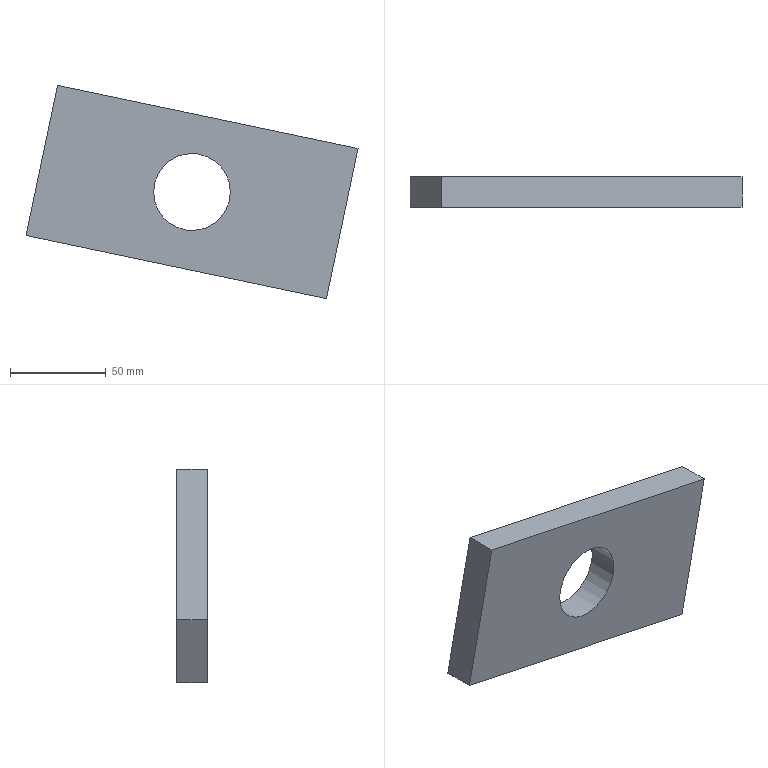Part | STEP file | 5_ESTAGIO_005 | 1 solid | 7 faces | box 173.032 x 16 x 111.193 mm | volume 184694 mm3 | plane 6 | cylinder 1 | commonest cylinder face diameters 40 x1
STEP:
#1=CARTESIAN_POINT('',(0.,0.,0.));
#2=DIRECTION('',(0.,0.,1.));
#3=DIRECTION('',(1.,0.,0.));
#4=AXIS2_PLACEMENT_3D('',#1,#2,#3);
#5=CARTESIAN_POINT('',(-2623.456,-962.15,953.739));
#6=VERTEX_POINT('',#5);
#7=CARTESIAN_POINT('',(-2641.008,-962.15,963.327));
#8=DIRECTION('',(0.,1.,0.));
#9=DIRECTION('',(1.,0.,0.));
#10=AXIS2_PLACEMENT_3D('',#7,#8,#9);
#11=CIRCLE('',#10,20.);
#12=CARTESIAN_POINT('',(-2641.008,-962.05,963.327));
#13=DIRECTION('',(0.,1.,0.));
#14=DIRECTION('',(0.8776,0.,-0.4794));
#15=AXIS2_PLACEMENT_3D('',#12,#13,#14);
#16=CYLINDRICAL_SURFACE('',#15,20.);
#17=CARTESIAN_POINT('',(-0.5,-0.1));
#18=DIRECTION('',(1.,0.));
#19=VECTOR('',#18,1.);
#20=LINE('',#17,#19);
#21=(GEOMETRIC_REPRESENTATION_CONTEXT(2)PARAMETRIC_REPRESENTATION_CONTEXT()REPRESENTATION_CONTEXT('',''));
#22=DEFINITIONAL_REPRESENTATION('',(#20),#21);
#23=PCURVE('',#16,#22);
#24=CARTESIAN_POINT('',(0.,-962.15,0.));
#25=DIRECTION('',(0.,1.,0.));
#26=DIRECTION('',(0.,0.,1.));
#27=AXIS2_PLACEMENT_3D('',#24,#25,#26);
#28=PLANE('',#27);
#29=CARTESIAN_POINT('',(963.327,-2641.008));
#30=DIRECTION('',(0.,1.));
#31=AXIS2_PLACEMENT_2D('',#29,#30);
#32=CIRCLE('',#31,20.);
#33=(GEOMETRIC_REPRESENTATION_CONTEXT(2)PARAMETRIC_REPRESENTATION_CONTEXT()REPRESENTATION_CONTEXT('',''));
#34=DEFINITIONAL_REPRESENTATION('',(#32),#33);
#35=PCURVE('',#28,#34);
#36=SURFACE_CURVE('',#11,(#23,#35),.PCURVE_S1.);
#37=EDGE_CURVE('',#6,#6,#36,.T.);
#38=ORIENTED_EDGE('',*,*,#37,.T.);
#39=CARTESIAN_POINT('',(-2623.456,-946.15,953.739));
#40=VERTEX_POINT('',#39);
#41=CARTESIAN_POINT('',(-2623.456,-962.15,953.739));
#42=CARTESIAN_POINT('',(-2623.456,-946.15,953.739));
#43=B_SPLINE_CURVE_WITH_KNOTS('',1,(#41,#42),.UNSPECIFIED.,.F.,.F.,(2,2),(-0.1,15.9),.PIECEWISE_BEZIER_KNOTS.);
#44=CARTESIAN_POINT('',(6.283,0.));
#45=DIRECTION('',(0.,1.));
#46=VECTOR('',#45,1.);
#47=LINE('',#44,#46);
#48=(GEOMETRIC_REPRESENTATION_CONTEXT(2)PARAMETRIC_REPRESENTATION_CONTEXT()REPRESENTATION_CONTEXT('',''));
#49=DEFINITIONAL_REPRESENTATION('',(#47),#48);
#50=PCURVE('',#16,#49);
#51=CARTESIAN_POINT('',(0.,0.));
#52=DIRECTION('',(0.,1.));
#53=VECTOR('',#52,1.);
#54=LINE('',#51,#53);
#55=(GEOMETRIC_REPRESENTATION_CONTEXT(2)PARAMETRIC_REPRESENTATION_CONTEXT()REPRESENTATION_CONTEXT('',''));
#56=DEFINITIONAL_REPRESENTATION('',(#54),#55);
#57=PCURVE('',#16,#56);
#58=SEAM_CURVE('',#43,(#50,#57),.PCURVE_S1.);
#59=EDGE_CURVE('',#6,#40,#58,.T.);
#60=ORIENTED_EDGE('',*,*,#59,.T.);
#61=CARTESIAN_POINT('',(-2641.008,-946.15,963.327));
#62=DIRECTION('',(0.,1.,0.));
#63=DIRECTION('',(1.,0.,0.));
#64=AXIS2_PLACEMENT_3D('',#61,#62,#63);
#65=CIRCLE('',#64,20.);
#66=CARTESIAN_POINT('',(-0.5,15.9));
#67=DIRECTION('',(1.,0.));
#68=VECTOR('',#67,1.);
#69=LINE('',#66,#68);
#70=(GEOMETRIC_REPRESENTATION_CONTEXT(2)PARAMETRIC_REPRESENTATION_CONTEXT()REPRESENTATION_CONTEXT('',''));
#71=DEFINITIONAL_REPRESENTATION('',(#69),#70);
#72=PCURVE('',#16,#71);
#73=CARTESIAN_POINT('',(0.,-946.15,0.));
#74=DIRECTION('',(0.,1.,0.));
#75=DIRECTION('',(0.,0.,1.));
#76=AXIS2_PLACEMENT_3D('',#73,#74,#75);
#77=PLANE('',#76);
#78=CARTESIAN_POINT('',(963.327,-2641.008));
#79=DIRECTION('',(0.,1.));
#80=AXIS2_PLACEMENT_2D('',#78,#79);
#81=CIRCLE('',#80,20.);
#82=(GEOMETRIC_REPRESENTATION_CONTEXT(2)PARAMETRIC_REPRESENTATION_CONTEXT()REPRESENTATION_CONTEXT('',''));
#83=DEFINITIONAL_REPRESENTATION('',(#81),#82);
#84=PCURVE('',#77,#83);
#85=SURFACE_CURVE('',#65,(#72,#84),.PCURVE_S1.);
#86=EDGE_CURVE('',#40,#40,#85,.T.);
#87=ORIENTED_EDGE('',*,*,#86,.F.);
#88=ORIENTED_EDGE('',*,*,#59,.F.);
#89=EDGE_LOOP('',(#38,#60,#87,#88));
#90=FACE_BOUND('',#89,.F.);
#91=ADVANCED_FACE('',(#90),#16,.F.);
#92=CARTESIAN_POINT('',(-2570.943,-946.15,907.731));
#93=VERTEX_POINT('',#92);
#94=CARTESIAN_POINT('',(-2554.492,-946.15,986.021));
#95=VERTEX_POINT('',#94);
#96=CARTESIAN_POINT('',(-2570.943,-946.15,907.731));
#97=DIRECTION('',(0.2056,0.,0.9786));
#98=VECTOR('',#97,1.);
#99=LINE('',#96,#98);
#100=CARTESIAN_POINT('',(907.731,-2570.943));
#101=DIRECTION('',(0.9786,0.2056));
#102=VECTOR('',#101,1.);
#103=LINE('',#100,#102);
#104=(GEOMETRIC_REPRESENTATION_CONTEXT(2)PARAMETRIC_REPRESENTATION_CONTEXT()REPRESENTATION_CONTEXT('',''));
#105=DEFINITIONAL_REPRESENTATION('',(#103),#104);
#106=PCURVE('',#77,#105);
#107=CARTESIAN_POINT('',(-2570.943,-946.15,907.731));
#108=DIRECTION('',(0.9786,0.,-0.2056));
#109=DIRECTION('',(-0.2056,0.,-0.9786));
#110=AXIS2_PLACEMENT_3D('',#107,#108,#109);
#111=PLANE('',#110);
#112=CARTESIAN_POINT('',(0.,0.));
#113=DIRECTION('',(-1.,0.));
#114=VECTOR('',#113,1.);
#115=LINE('',#112,#114);
#116=(GEOMETRIC_REPRESENTATION_CONTEXT(2)PARAMETRIC_REPRESENTATION_CONTEXT()REPRESENTATION_CONTEXT('',''));
#117=DEFINITIONAL_REPRESENTATION('',(#115),#116);
#118=PCURVE('',#111,#117);
#119=SURFACE_CURVE('',#99,(#106,#118),.PCURVE_S1.);
#120=EDGE_CURVE('',#93,#95,#119,.T.);
#121=ORIENTED_EDGE('',*,*,#120,.F.);
#122=CARTESIAN_POINT('',(-2727.523,-946.15,940.634));
#123=VERTEX_POINT('',#122);
#124=CARTESIAN_POINT('',(-2727.523,-946.15,940.634));
#125=DIRECTION('',(0.9786,0.,-0.2056));
#126=VECTOR('',#125,1.);
#127=LINE('',#124,#126);
#128=CARTESIAN_POINT('',(940.634,-2727.523));
#129=DIRECTION('',(-0.2056,0.9786));
#130=VECTOR('',#129,1.);
#131=LINE('',#128,#130);
#132=(GEOMETRIC_REPRESENTATION_CONTEXT(2)PARAMETRIC_REPRESENTATION_CONTEXT()REPRESENTATION_CONTEXT('',''));
#133=DEFINITIONAL_REPRESENTATION('',(#131),#132);
#134=PCURVE('',#77,#133);
#135=CARTESIAN_POINT('',(-2727.523,-946.15,940.634));
#136=DIRECTION('',(-0.2056,0.,-0.9786));
#137=DIRECTION('',(-0.9786,0.,0.2056));
#138=AXIS2_PLACEMENT_3D('',#135,#136,#137);
#139=PLANE('',#138);
#140=CARTESIAN_POINT('',(0.000000002,0.));
#141=DIRECTION('',(-1.,0.));
#142=VECTOR('',#141,1.);
#143=LINE('',#140,#142);
#144=(GEOMETRIC_REPRESENTATION_CONTEXT(2)PARAMETRIC_REPRESENTATION_CONTEXT()REPRESENTATION_CONTEXT('',''));
#145=DEFINITIONAL_REPRESENTATION('',(#143),#144);
#146=PCURVE('',#139,#145);
#147=SURFACE_CURVE('',#127,(#134,#146),.PCURVE_S1.);
#148=EDGE_CURVE('',#123,#93,#147,.T.);
#149=ORIENTED_EDGE('',*,*,#148,.F.);
#150=CARTESIAN_POINT('',(-2711.072,-946.15,1018.924));
#151=VERTEX_POINT('',#150);
#152=CARTESIAN_POINT('',(-2711.072,-946.15,1018.924));
#153=DIRECTION('',(-0.2056,0.,-0.9786));
#154=VECTOR('',#153,1.);
#155=LINE('',#152,#154);
#156=CARTESIAN_POINT('',(1018.924,-2711.072));
#157=DIRECTION('',(-0.9786,-0.2056));
#158=VECTOR('',#157,1.);
#159=LINE('',#156,#158);
#160=(GEOMETRIC_REPRESENTATION_CONTEXT(2)PARAMETRIC_REPRESENTATION_CONTEXT()REPRESENTATION_CONTEXT('',''));
#161=DEFINITIONAL_REPRESENTATION('',(#159),#160);
#162=PCURVE('',#77,#161);
#163=CARTESIAN_POINT('',(-2711.072,-946.15,1018.924));
#164=DIRECTION('',(-0.9786,0.,0.2056));
#165=DIRECTION('',(0.2056,0.,0.9786));
#166=AXIS2_PLACEMENT_3D('',#163,#164,#165);
#167=PLANE('',#166);
#168=CARTESIAN_POINT('',(-0.000000001,0.));
#169=DIRECTION('',(-1.,0.));
#170=VECTOR('',#169,1.);
#171=LINE('',#168,#170);
#172=(GEOMETRIC_REPRESENTATION_CONTEXT(2)PARAMETRIC_REPRESENTATION_CONTEXT()REPRESENTATION_CONTEXT('',''));
#173=DEFINITIONAL_REPRESENTATION('',(#171),#172);
#174=PCURVE('',#167,#173);
#175=SURFACE_CURVE('',#155,(#162,#174),.PCURVE_S1.);
#176=EDGE_CURVE('',#151,#123,#175,.T.);
#177=ORIENTED_EDGE('',*,*,#176,.F.);
#178=CARTESIAN_POINT('',(-2554.492,-946.15,986.021));
#179=DIRECTION('',(-0.9786,0.,0.2056));
#180=VECTOR('',#179,1.);
#181=LINE('',#178,#180);
#182=CARTESIAN_POINT('',(986.021,-2554.492));
#183=DIRECTION('',(0.2056,-0.9786));
#184=VECTOR('',#183,1.);
#185=LINE('',#182,#184);
#186=(GEOMETRIC_REPRESENTATION_CONTEXT(2)PARAMETRIC_REPRESENTATION_CONTEXT()REPRESENTATION_CONTEXT('',''));
#187=DEFINITIONAL_REPRESENTATION('',(#185),#186);
#188=PCURVE('',#77,#187);
#189=CARTESIAN_POINT('',(-2554.492,-946.15,986.021));
#190=DIRECTION('',(0.2056,0.,0.9786));
#191=DIRECTION('',(0.9786,0.,-0.2056));
#192=AXIS2_PLACEMENT_3D('',#189,#190,#191);
#193=PLANE('',#192);
#194=CARTESIAN_POINT('',(0.000000002,0.));
#195=DIRECTION('',(-1.,0.));
#196=VECTOR('',#195,1.);
#197=LINE('',#194,#196);
#198=(GEOMETRIC_REPRESENTATION_CONTEXT(2)PARAMETRIC_REPRESENTATION_CONTEXT()REPRESENTATION_CONTEXT('',''));
#199=DEFINITIONAL_REPRESENTATION('',(#197),#198);
#200=PCURVE('',#193,#199);
#201=SURFACE_CURVE('',#181,(#188,#200),.PCURVE_S1.);
#202=EDGE_CURVE('',#95,#151,#201,.T.);
#203=ORIENTED_EDGE('',*,*,#202,.F.);
#204=EDGE_LOOP('',(#121,#149,#177,#203));
#205=FACE_BOUND('',#204,.T.);
#206=ORIENTED_EDGE('',*,*,#86,.F.);
#207=EDGE_LOOP('',(#206));
#208=FACE_BOUND('',#207,.T.);
#209=ADVANCED_FACE('',(#205,#208),#77,.T.);
#210=CARTESIAN_POINT('',(-2570.943,-962.15,907.731));
#211=VERTEX_POINT('',#210);
#212=CARTESIAN_POINT('',(-2554.492,-962.15,986.021));
#213=VERTEX_POINT('',#212);
#214=CARTESIAN_POINT('',(-2570.943,-962.15,907.731));
#215=DIRECTION('',(0.2056,0.,0.9786));
#216=VECTOR('',#215,1.);
#217=LINE('',#214,#216);
#218=CARTESIAN_POINT('',(0.,-16.));
#219=DIRECTION('',(-1.,0.));
#220=VECTOR('',#219,1.);
#221=LINE('',#218,#220);
#222=(GEOMETRIC_REPRESENTATION_CONTEXT(2)PARAMETRIC_REPRESENTATION_CONTEXT()REPRESENTATION_CONTEXT('',''));
#223=DEFINITIONAL_REPRESENTATION('',(#221),#222);
#224=PCURVE('',#111,#223);
#225=CARTESIAN_POINT('',(907.731,-2570.943));
#226=DIRECTION('',(0.9786,0.2056));
#227=VECTOR('',#226,1.);
#228=LINE('',#225,#227);
#229=(GEOMETRIC_REPRESENTATION_CONTEXT(2)PARAMETRIC_REPRESENTATION_CONTEXT()REPRESENTATION_CONTEXT('',''));
#230=DEFINITIONAL_REPRESENTATION('',(#228),#229);
#231=PCURVE('',#28,#230);
#232=SURFACE_CURVE('',#217,(#224,#231),.PCURVE_S1.);
#233=EDGE_CURVE('',#211,#213,#232,.T.);
#234=ORIENTED_EDGE('',*,*,#233,.F.);
#235=CARTESIAN_POINT('',(-2570.943,-946.15,907.731));
#236=DIRECTION('',(0.,-1.,0.));
#237=VECTOR('',#236,1.);
#238=LINE('',#235,#237);
#239=CARTESIAN_POINT('',(0.,0.));
#240=DIRECTION('',(0.,-1.));
#241=VECTOR('',#240,1.);
#242=LINE('',#239,#241);
#243=(GEOMETRIC_REPRESENTATION_CONTEXT(2)PARAMETRIC_REPRESENTATION_CONTEXT()REPRESENTATION_CONTEXT('',''));
#244=DEFINITIONAL_REPRESENTATION('',(#242),#243);
#245=PCURVE('',#111,#244);
#246=CARTESIAN_POINT('',(-160.,0.));
#247=DIRECTION('',(0.,-1.));
#248=VECTOR('',#247,1.);
#249=LINE('',#246,#248);
#250=(GEOMETRIC_REPRESENTATION_CONTEXT(2)PARAMETRIC_REPRESENTATION_CONTEXT()REPRESENTATION_CONTEXT('',''));
#251=DEFINITIONAL_REPRESENTATION('',(#249),#250);
#252=PCURVE('',#139,#251);
#253=SURFACE_CURVE('',#238,(#245,#252),.PCURVE_S1.);
#254=EDGE_CURVE('',#93,#211,#253,.T.);
#255=ORIENTED_EDGE('',*,*,#254,.F.);
#256=ORIENTED_EDGE('',*,*,#120,.T.);
#257=CARTESIAN_POINT('',(-2554.492,-946.15,986.021));
#258=DIRECTION('',(0.,-1.,0.));
#259=VECTOR('',#258,1.);
#260=LINE('',#257,#259);
#261=CARTESIAN_POINT('',(-80.,0.));
#262=DIRECTION('',(0.,-1.));
#263=VECTOR('',#262,1.);
#264=LINE('',#261,#263);
#265=(GEOMETRIC_REPRESENTATION_CONTEXT(2)PARAMETRIC_REPRESENTATION_CONTEXT()REPRESENTATION_CONTEXT('',''));
#266=DEFINITIONAL_REPRESENTATION('',(#264),#265);
#267=PCURVE('',#111,#266);
#268=CARTESIAN_POINT('',(0.,0.));
#269=DIRECTION('',(0.,-1.));
#270=VECTOR('',#269,1.);
#271=LINE('',#268,#270);
#272=(GEOMETRIC_REPRESENTATION_CONTEXT(2)PARAMETRIC_REPRESENTATION_CONTEXT()REPRESENTATION_CONTEXT('',''));
#273=DEFINITIONAL_REPRESENTATION('',(#271),#272);
#274=PCURVE('',#193,#273);
#275=SURFACE_CURVE('',#260,(#267,#274),.PCURVE_S1.);
#276=EDGE_CURVE('',#95,#213,#275,.T.);
#277=ORIENTED_EDGE('',*,*,#276,.T.);
#278=EDGE_LOOP('',(#234,#255,#256,#277));
#279=FACE_BOUND('',#278,.T.);
#280=ADVANCED_FACE('',(#279),#111,.T.);
#281=CARTESIAN_POINT('',(-2727.523,-962.15,940.634));
#282=VERTEX_POINT('',#281);
#283=CARTESIAN_POINT('',(-2727.523,-962.15,940.634));
#284=DIRECTION('',(0.9786,0.,-0.2056));
#285=VECTOR('',#284,1.);
#286=LINE('',#283,#285);
#287=CARTESIAN_POINT('',(0.000000002,-16.));
#288=DIRECTION('',(-1.,0.));
#289=VECTOR('',#288,1.);
#290=LINE('',#287,#289);
#291=(GEOMETRIC_REPRESENTATION_CONTEXT(2)PARAMETRIC_REPRESENTATION_CONTEXT()REPRESENTATION_CONTEXT('',''));
#292=DEFINITIONAL_REPRESENTATION('',(#290),#291);
#293=PCURVE('',#139,#292);
#294=CARTESIAN_POINT('',(940.634,-2727.523));
#295=DIRECTION('',(-0.2056,0.9786));
#296=VECTOR('',#295,1.);
#297=LINE('',#294,#296);
#298=(GEOMETRIC_REPRESENTATION_CONTEXT(2)PARAMETRIC_REPRESENTATION_CONTEXT()REPRESENTATION_CONTEXT('',''));
#299=DEFINITIONAL_REPRESENTATION('',(#297),#298);
#300=PCURVE('',#28,#299);
#301=SURFACE_CURVE('',#286,(#293,#300),.PCURVE_S1.);
#302=EDGE_CURVE('',#282,#211,#301,.T.);
#303=ORIENTED_EDGE('',*,*,#302,.F.);
#304=CARTESIAN_POINT('',(-2727.523,-946.15,940.634));
#305=DIRECTION('',(0.,-1.,0.));
#306=VECTOR('',#305,1.);
#307=LINE('',#304,#306);
#308=CARTESIAN_POINT('',(0.,0.));
#309=DIRECTION('',(0.,-1.));
#310=VECTOR('',#309,1.);
#311=LINE('',#308,#310);
#312=(GEOMETRIC_REPRESENTATION_CONTEXT(2)PARAMETRIC_REPRESENTATION_CONTEXT()REPRESENTATION_CONTEXT('',''));
#313=DEFINITIONAL_REPRESENTATION('',(#311),#312);
#314=PCURVE('',#139,#313);
#315=CARTESIAN_POINT('',(-80.,0.));
#316=DIRECTION('',(0.,-1.));
#317=VECTOR('',#316,1.);
#318=LINE('',#315,#317);
#319=(GEOMETRIC_REPRESENTATION_CONTEXT(2)PARAMETRIC_REPRESENTATION_CONTEXT()REPRESENTATION_CONTEXT('',''));
#320=DEFINITIONAL_REPRESENTATION('',(#318),#319);
#321=PCURVE('',#167,#320);
#322=SURFACE_CURVE('',#307,(#314,#321),.PCURVE_S1.);
#323=EDGE_CURVE('',#123,#282,#322,.T.);
#324=ORIENTED_EDGE('',*,*,#323,.F.);
#325=ORIENTED_EDGE('',*,*,#148,.T.);
#326=ORIENTED_EDGE('',*,*,#254,.T.);
#327=EDGE_LOOP('',(#303,#324,#325,#326));
#328=FACE_BOUND('',#327,.T.);
#329=ADVANCED_FACE('',(#328),#139,.T.);
#330=CARTESIAN_POINT('',(-2711.072,-962.15,1018.924));
#331=VERTEX_POINT('',#330);
#332=CARTESIAN_POINT('',(-2711.072,-962.15,1018.924));
#333=DIRECTION('',(-0.2056,0.,-0.9786));
#334=VECTOR('',#333,1.);
#335=LINE('',#332,#334);
#336=CARTESIAN_POINT('',(-0.000000001,-16.));
#337=DIRECTION('',(-1.,0.));
#338=VECTOR('',#337,1.);
#339=LINE('',#336,#338);
#340=(GEOMETRIC_REPRESENTATION_CONTEXT(2)PARAMETRIC_REPRESENTATION_CONTEXT()REPRESENTATION_CONTEXT('',''));
#341=DEFINITIONAL_REPRESENTATION('',(#339),#340);
#342=PCURVE('',#167,#341);
#343=CARTESIAN_POINT('',(1018.924,-2711.072));
#344=DIRECTION('',(-0.9786,-0.2056));
#345=VECTOR('',#344,1.);
#346=LINE('',#343,#345);
#347=(GEOMETRIC_REPRESENTATION_CONTEXT(2)PARAMETRIC_REPRESENTATION_CONTEXT()REPRESENTATION_CONTEXT('',''));
#348=DEFINITIONAL_REPRESENTATION('',(#346),#347);
#349=PCURVE('',#28,#348);
#350=SURFACE_CURVE('',#335,(#342,#349),.PCURVE_S1.);
#351=EDGE_CURVE('',#331,#282,#350,.T.);
#352=ORIENTED_EDGE('',*,*,#351,.F.);
#353=CARTESIAN_POINT('',(-2711.072,-946.15,1018.924));
#354=DIRECTION('',(0.,-1.,0.));
#355=VECTOR('',#354,1.);
#356=LINE('',#353,#355);
#357=CARTESIAN_POINT('',(0.,0.));
#358=DIRECTION('',(0.,-1.));
#359=VECTOR('',#358,1.);
#360=LINE('',#357,#359);
#361=(GEOMETRIC_REPRESENTATION_CONTEXT(2)PARAMETRIC_REPRESENTATION_CONTEXT()REPRESENTATION_CONTEXT('',''));
#362=DEFINITIONAL_REPRESENTATION('',(#360),#361);
#363=PCURVE('',#167,#362);
#364=CARTESIAN_POINT('',(-160.,0.));
#365=DIRECTION('',(0.,-1.));
#366=VECTOR('',#365,1.);
#367=LINE('',#364,#366);
#368=(GEOMETRIC_REPRESENTATION_CONTEXT(2)PARAMETRIC_REPRESENTATION_CONTEXT()REPRESENTATION_CONTEXT('',''));
#369=DEFINITIONAL_REPRESENTATION('',(#367),#368);
#370=PCURVE('',#193,#369);
#371=SURFACE_CURVE('',#356,(#363,#370),.PCURVE_S1.);
#372=EDGE_CURVE('',#151,#331,#371,.T.);
#373=ORIENTED_EDGE('',*,*,#372,.F.);
#374=ORIENTED_EDGE('',*,*,#176,.T.);
#375=ORIENTED_EDGE('',*,*,#323,.T.);
#376=EDGE_LOOP('',(#352,#373,#374,#375));
#377=FACE_BOUND('',#376,.T.);
#378=ADVANCED_FACE('',(#377),#167,.T.);
#379=CARTESIAN_POINT('',(-2554.492,-962.15,986.021));
#380=DIRECTION('',(-0.9786,0.,0.2056));
#381=VECTOR('',#380,1.);
#382=LINE('',#379,#381);
#383=CARTESIAN_POINT('',(0.000000002,-16.));
#384=DIRECTION('',(-1.,0.));
#385=VECTOR('',#384,1.);
#386=LINE('',#383,#385);
#387=(GEOMETRIC_REPRESENTATION_CONTEXT(2)PARAMETRIC_REPRESENTATION_CONTEXT()REPRESENTATION_CONTEXT('',''));
#388=DEFINITIONAL_REPRESENTATION('',(#386),#387);
#389=PCURVE('',#193,#388);
#390=CARTESIAN_POINT('',(986.021,-2554.492));
#391=DIRECTION('',(0.2056,-0.9786));
#392=VECTOR('',#391,1.);
#393=LINE('',#390,#392);
#394=(GEOMETRIC_REPRESENTATION_CONTEXT(2)PARAMETRIC_REPRESENTATION_CONTEXT()REPRESENTATION_CONTEXT('',''));
#395=DEFINITIONAL_REPRESENTATION('',(#393),#394);
#396=PCURVE('',#28,#395);
#397=SURFACE_CURVE('',#382,(#389,#396),.PCURVE_S1.);
#398=EDGE_CURVE('',#213,#331,#397,.T.);
#399=ORIENTED_EDGE('',*,*,#398,.F.);
#400=ORIENTED_EDGE('',*,*,#276,.F.);
#401=ORIENTED_EDGE('',*,*,#202,.T.);
#402=ORIENTED_EDGE('',*,*,#372,.T.);
#403=EDGE_LOOP('',(#399,#400,#401,#402));
#404=FACE_BOUND('',#403,.T.);
#405=ADVANCED_FACE('',(#404),#193,.T.);
#406=ORIENTED_EDGE('',*,*,#398,.T.);
#407=ORIENTED_EDGE('',*,*,#351,.T.);
#408=ORIENTED_EDGE('',*,*,#302,.T.);
#409=ORIENTED_EDGE('',*,*,#233,.T.);
#410=EDGE_LOOP('',(#406,#407,#408,#409));
#411=FACE_BOUND('',#410,.T.);
#412=ORIENTED_EDGE('',*,*,#37,.T.);
#413=EDGE_LOOP('',(#412));
#414=FACE_BOUND('',#413,.T.);
#415=ADVANCED_FACE('',(#411,#414),#28,.F.);
#416=CLOSED_SHELL('',(#91,#209,#280,#329,#378,#405,#415));
#417=MANIFOLD_SOLID_BREP('',#416);
#418=(LENGTH_UNIT()NAMED_UNIT(*)SI_UNIT(.MILLI.,.METRE.));
#419=UNCERTAINTY_MEASURE_WITH_UNIT(LENGTH_MEASURE(0.000002),#418,'','');
#420=(NAMED_UNIT(*)PLANE_ANGLE_UNIT()SI_UNIT($,.RADIAN.));
#421=(NAMED_UNIT(*)SI_UNIT($,.STERADIAN.)SOLID_ANGLE_UNIT());
#422=(GEOMETRIC_REPRESENTATION_CONTEXT(3)GLOBAL_UNCERTAINTY_ASSIGNED_CONTEXT((#419))GLOBAL_UNIT_ASSIGNED_CONTEXT((#418,#420,#421))REPRESENTATION_CONTEXT('',''));
#423=ADVANCED_BREP_SHAPE_REPRESENTATION('',(#4,#417),#422);